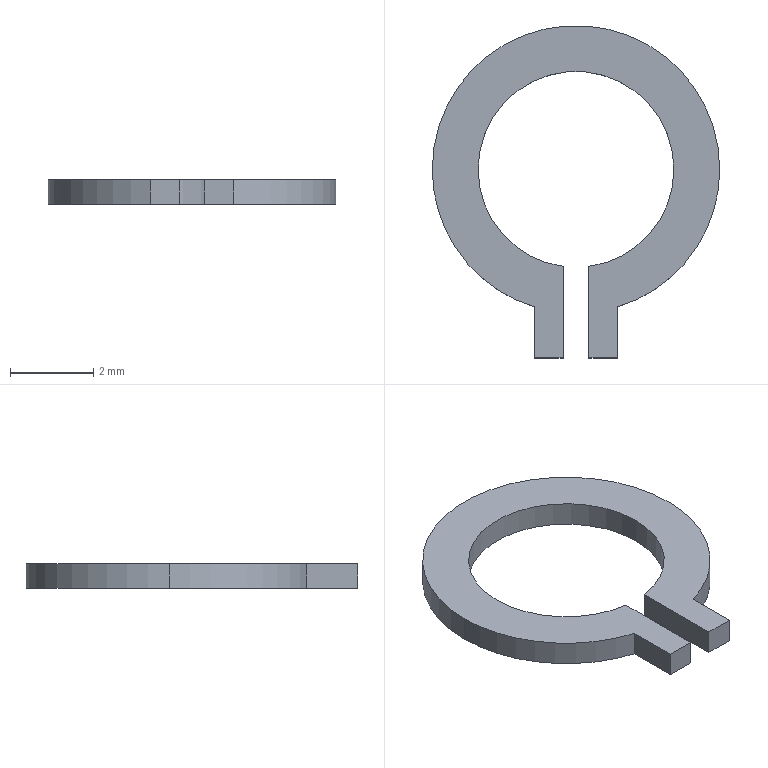Part | NX | 1 solid | 14 faces | box 6.9 x 7.977 x 0.6 mm | volume 12.565 mm3 | plane 8 | cylinder 6 | commonest cylinder face diameters 4.7 x3 6.9 x3
STEP:
#1=CARTESIAN_POINT('',(-1.,-4.527,0.));
#2=VERTEX_POINT('',#1);
#3=CARTESIAN_POINT('',(-1.,-3.302,0.));
#4=VERTEX_POINT('',#3);
#5=CARTESIAN_POINT('',(-1.,-4.527,0.));
#6=DIRECTION('',(0.,1.,0.));
#7=VECTOR('',#6,1000.);
#8=LINE('',#5,#7);
#9=EDGE_CURVE('',#2,#4,#8,.T.);
#10=ORIENTED_EDGE('',*,*,#9,.T.);
#11=CARTESIAN_POINT('',(-3.45,0.,0.));
#12=VERTEX_POINT('',#11);
#13=CARTESIAN_POINT('',(0.,0.,0.));
#14=DIRECTION('',(0.,0.,1.));
#15=DIRECTION('',(-1.,0.,0.));
#16=AXIS2_PLACEMENT_3D('',#13,#14,#15);
#17=CIRCLE('',#16,3.45);
#18=EDGE_CURVE('',#12,#4,#17,.T.);
#19=ORIENTED_EDGE('',*,*,#18,.F.);
#20=CARTESIAN_POINT('',(3.45,0.,0.));
#21=VERTEX_POINT('',#20);
#22=CARTESIAN_POINT('',(0.,0.,0.));
#23=DIRECTION('',(0.,0.,1.));
#24=DIRECTION('',(-1.,0.,0.));
#25=AXIS2_PLACEMENT_3D('',#22,#23,#24);
#26=CIRCLE('',#25,3.45);
#27=EDGE_CURVE('',#21,#12,#26,.T.);
#28=ORIENTED_EDGE('',*,*,#27,.F.);
#29=CARTESIAN_POINT('',(1.,-3.302,0.));
#30=VERTEX_POINT('',#29);
#31=CARTESIAN_POINT('',(0.,0.,0.));
#32=DIRECTION('',(0.,0.,1.));
#33=DIRECTION('',(-1.,0.,0.));
#34=AXIS2_PLACEMENT_3D('',#31,#32,#33);
#35=CIRCLE('',#34,3.45);
#36=EDGE_CURVE('',#30,#21,#35,.T.);
#37=ORIENTED_EDGE('',*,*,#36,.F.);
#38=CARTESIAN_POINT('',(1.,-4.527,0.));
#39=VERTEX_POINT('',#38);
#40=CARTESIAN_POINT('',(1.,-3.302,0.));
#41=DIRECTION('',(0.,-1.,0.));
#42=VECTOR('',#41,1000.);
#43=LINE('',#40,#42);
#44=EDGE_CURVE('',#30,#39,#43,.T.);
#45=ORIENTED_EDGE('',*,*,#44,.T.);
#46=CARTESIAN_POINT('',(0.31,-4.527,0.));
#47=VERTEX_POINT('',#46);
#48=CARTESIAN_POINT('',(1.,-4.527,0.));
#49=DIRECTION('',(-1.,0.,0.));
#50=VECTOR('',#49,1000.);
#51=LINE('',#48,#50);
#52=EDGE_CURVE('',#39,#47,#51,.T.);
#53=ORIENTED_EDGE('',*,*,#52,.T.);
#54=CARTESIAN_POINT('',(0.31,-2.329,0.));
#55=VERTEX_POINT('',#54);
#56=CARTESIAN_POINT('',(0.31,-4.527,0.));
#57=DIRECTION('',(0.,1.,0.));
#58=VECTOR('',#57,1000.);
#59=LINE('',#56,#58);
#60=EDGE_CURVE('',#47,#55,#59,.T.);
#61=ORIENTED_EDGE('',*,*,#60,.T.);
#62=CARTESIAN_POINT('',(2.35,0.,0.));
#63=VERTEX_POINT('',#62);
#64=CARTESIAN_POINT('',(0.,0.,0.));
#65=DIRECTION('',(0.,0.,-1.));
#66=DIRECTION('',(1.,0.,0.));
#67=AXIS2_PLACEMENT_3D('',#64,#65,#66);
#68=CIRCLE('',#67,2.35);
#69=EDGE_CURVE('',#63,#55,#68,.T.);
#70=ORIENTED_EDGE('',*,*,#69,.F.);
#71=CARTESIAN_POINT('',(-2.35,0.,0.));
#72=VERTEX_POINT('',#71);
#73=CARTESIAN_POINT('',(0.,0.,0.));
#74=DIRECTION('',(0.,0.,-1.));
#75=DIRECTION('',(1.,0.,0.));
#76=AXIS2_PLACEMENT_3D('',#73,#74,#75);
#77=CIRCLE('',#76,2.35);
#78=EDGE_CURVE('',#72,#63,#77,.T.);
#79=ORIENTED_EDGE('',*,*,#78,.F.);
#80=CARTESIAN_POINT('',(-0.31,-2.329,0.));
#81=VERTEX_POINT('',#80);
#82=CARTESIAN_POINT('',(0.,0.,0.));
#83=DIRECTION('',(0.,0.,-1.));
#84=DIRECTION('',(1.,0.,0.));
#85=AXIS2_PLACEMENT_3D('',#82,#83,#84);
#86=CIRCLE('',#85,2.35);
#87=EDGE_CURVE('',#81,#72,#86,.T.);
#88=ORIENTED_EDGE('',*,*,#87,.F.);
#89=CARTESIAN_POINT('',(-0.31,-4.527,0.));
#90=VERTEX_POINT('',#89);
#91=CARTESIAN_POINT('',(-0.31,-2.329,0.));
#92=DIRECTION('',(0.,-1.,0.));
#93=VECTOR('',#92,1000.);
#94=LINE('',#91,#93);
#95=EDGE_CURVE('',#81,#90,#94,.T.);
#96=ORIENTED_EDGE('',*,*,#95,.T.);
#97=CARTESIAN_POINT('',(-0.31,-4.527,0.));
#98=DIRECTION('',(-1.,0.,0.));
#99=VECTOR('',#98,1000.);
#100=LINE('',#97,#99);
#101=EDGE_CURVE('',#90,#2,#100,.T.);
#102=ORIENTED_EDGE('',*,*,#101,.T.);
#103=EDGE_LOOP('',(#10,#19,#28,#37,#45,#53,#61,#70,#79,#88,#96,#102));
#104=FACE_BOUND('',#103,.T.);
#105=CARTESIAN_POINT('',(0.,0.,0.));
#106=DIRECTION('',(0.,0.,1.));
#107=DIRECTION('',(1.,0.,0.));
#108=AXIS2_PLACEMENT_3D('',#105,#106,#107);
#109=PLANE('',#108);
#110=ADVANCED_FACE('',(#104),#109,.F.);
#111=ORIENTED_EDGE('',*,*,#9,.F.);
#112=CARTESIAN_POINT('',(-1.,-4.527,0.6));
#113=VERTEX_POINT('',#112);
#114=CARTESIAN_POINT('',(-1.,-4.527,0.6));
#115=DIRECTION('',(0.,0.,-1.));
#116=VECTOR('',#115,1000.);
#117=LINE('',#114,#116);
#118=EDGE_CURVE('',#113,#2,#117,.T.);
#119=ORIENTED_EDGE('',*,*,#118,.F.);
#120=CARTESIAN_POINT('',(-1.,-3.302,0.6));
#121=VERTEX_POINT('',#120);
#122=CARTESIAN_POINT('',(-1.,-4.527,0.6));
#123=DIRECTION('',(0.,1.,0.));
#124=VECTOR('',#123,1000.);
#125=LINE('',#122,#124);
#126=EDGE_CURVE('',#113,#121,#125,.T.);
#127=ORIENTED_EDGE('',*,*,#126,.T.);
#128=CARTESIAN_POINT('',(-1.,-3.302,0.6));
#129=DIRECTION('',(0.,0.,-1.));
#130=VECTOR('',#129,1000.);
#131=LINE('',#128,#130);
#132=EDGE_CURVE('',#121,#4,#131,.T.);
#133=ORIENTED_EDGE('',*,*,#132,.T.);
#134=EDGE_LOOP('',(#111,#119,#127,#133));
#135=FACE_BOUND('',#134,.T.);
#136=CARTESIAN_POINT('',(-1.,-3.302,0.));
#137=DIRECTION('',(-1.,0.,0.));
#138=DIRECTION('',(0.,0.,1.));
#139=AXIS2_PLACEMENT_3D('',#136,#137,#138);
#140=PLANE('',#139);
#141=ADVANCED_FACE('',(#135),#140,.T.);
#142=CARTESIAN_POINT('',(-3.45,0.,0.6));
#143=VERTEX_POINT('',#142);
#144=CARTESIAN_POINT('',(-3.45,0.,0.));
#145=DIRECTION('',(0.,0.,1.));
#146=VECTOR('',#145,1000.);
#147=LINE('',#144,#146);
#148=EDGE_CURVE('',#12,#143,#147,.T.);
#149=ORIENTED_EDGE('',*,*,#148,.F.);
#150=ORIENTED_EDGE('',*,*,#18,.T.);
#151=ORIENTED_EDGE('',*,*,#132,.F.);
#152=CARTESIAN_POINT('',(0.,0.,0.6));
#153=DIRECTION('',(0.,0.,-1.));
#154=DIRECTION('',(-0.2899,-0.9571,0.));
#155=AXIS2_PLACEMENT_3D('',#152,#153,#154);
#156=CIRCLE('',#155,3.45);
#157=EDGE_CURVE('',#121,#143,#156,.T.);
#158=ORIENTED_EDGE('',*,*,#157,.T.);
#159=EDGE_LOOP('',(#149,#150,#151,#158));
#160=FACE_BOUND('',#159,.T.);
#161=CARTESIAN_POINT('',(0.,0.,0.));
#162=DIRECTION('',(0.,0.,1.));
#163=DIRECTION('',(1.,0.,0.));
#164=AXIS2_PLACEMENT_3D('',#161,#162,#163);
#165=CYLINDRICAL_SURFACE('',#164,3.45);
#166=ADVANCED_FACE('',(#160),#165,.T.);
#167=ORIENTED_EDGE('',*,*,#44,.F.);
#168=CARTESIAN_POINT('',(1.,-3.302,0.6));
#169=VERTEX_POINT('',#168);
#170=CARTESIAN_POINT('',(1.,-3.302,0.));
#171=DIRECTION('',(0.,0.,1.));
#172=VECTOR('',#171,1000.);
#173=LINE('',#170,#172);
#174=EDGE_CURVE('',#30,#169,#173,.T.);
#175=ORIENTED_EDGE('',*,*,#174,.T.);
#176=CARTESIAN_POINT('',(1.,-4.527,0.6));
#177=VERTEX_POINT('',#176);
#178=CARTESIAN_POINT('',(1.,-3.302,0.6));
#179=DIRECTION('',(0.,-1.,0.));
#180=VECTOR('',#179,1000.);
#181=LINE('',#178,#180);
#182=EDGE_CURVE('',#169,#177,#181,.T.);
#183=ORIENTED_EDGE('',*,*,#182,.T.);
#184=CARTESIAN_POINT('',(1.,-4.527,0.6));
#185=DIRECTION('',(0.,0.,-1.));
#186=VECTOR('',#185,1000.);
#187=LINE('',#184,#186);
#188=EDGE_CURVE('',#177,#39,#187,.T.);
#189=ORIENTED_EDGE('',*,*,#188,.T.);
#190=EDGE_LOOP('',(#167,#175,#183,#189));
#191=FACE_BOUND('',#190,.T.);
#192=CARTESIAN_POINT('',(1.,-4.527,0.));
#193=DIRECTION('',(1.,0.,0.));
#194=DIRECTION('',(0.,1.,0.));
#195=AXIS2_PLACEMENT_3D('',#192,#193,#194);
#196=PLANE('',#195);
#197=ADVANCED_FACE('',(#191),#196,.T.);
#198=ORIENTED_EDGE('',*,*,#52,.F.);
#199=ORIENTED_EDGE('',*,*,#188,.F.);
#200=CARTESIAN_POINT('',(0.31,-4.527,0.6));
#201=VERTEX_POINT('',#200);
#202=CARTESIAN_POINT('',(1.,-4.527,0.6));
#203=DIRECTION('',(-1.,0.,0.));
#204=VECTOR('',#203,1000.);
#205=LINE('',#202,#204);
#206=EDGE_CURVE('',#177,#201,#205,.T.);
#207=ORIENTED_EDGE('',*,*,#206,.T.);
#208=CARTESIAN_POINT('',(0.31,-4.527,0.6));
#209=DIRECTION('',(0.,0.,-1.));
#210=VECTOR('',#209,1000.);
#211=LINE('',#208,#210);
#212=EDGE_CURVE('',#201,#47,#211,.T.);
#213=ORIENTED_EDGE('',*,*,#212,.T.);
#214=EDGE_LOOP('',(#198,#199,#207,#213));
#215=FACE_BOUND('',#214,.T.);
#216=CARTESIAN_POINT('',(0.31,-4.527,0.));
#217=DIRECTION('',(0.,-1.,0.));
#218=DIRECTION('',(0.,0.,-1.));
#219=AXIS2_PLACEMENT_3D('',#216,#217,#218);
#220=PLANE('',#219);
#221=ADVANCED_FACE('',(#215),#220,.T.);
#222=ORIENTED_EDGE('',*,*,#60,.F.);
#223=ORIENTED_EDGE('',*,*,#212,.F.);
#224=CARTESIAN_POINT('',(0.31,-2.329,0.6));
#225=VERTEX_POINT('',#224);
#226=CARTESIAN_POINT('',(0.31,-4.527,0.6));
#227=DIRECTION('',(0.,1.,0.));
#228=VECTOR('',#227,1000.);
#229=LINE('',#226,#228);
#230=EDGE_CURVE('',#201,#225,#229,.T.);
#231=ORIENTED_EDGE('',*,*,#230,.T.);
#232=CARTESIAN_POINT('',(0.31,-2.329,0.6));
#233=DIRECTION('',(0.,0.,-1.));
#234=VECTOR('',#233,1000.);
#235=LINE('',#232,#234);
#236=EDGE_CURVE('',#225,#55,#235,.T.);
#237=ORIENTED_EDGE('',*,*,#236,.T.);
#238=EDGE_LOOP('',(#222,#223,#231,#237));
#239=FACE_BOUND('',#238,.T.);
#240=CARTESIAN_POINT('',(0.31,-2.329,0.));
#241=DIRECTION('',(-1.,0.,0.));
#242=DIRECTION('',(0.,0.,1.));
#243=AXIS2_PLACEMENT_3D('',#240,#241,#242);
#244=PLANE('',#243);
#245=ADVANCED_FACE('',(#239),#244,.T.);
#246=CARTESIAN_POINT('',(2.35,0.,0.6));
#247=VERTEX_POINT('',#246);
#248=CARTESIAN_POINT('',(2.35,0.,0.));
#249=DIRECTION('',(0.,0.,1.));
#250=VECTOR('',#249,1000.);
#251=LINE('',#248,#250);
#252=EDGE_CURVE('',#63,#247,#251,.T.);
#253=ORIENTED_EDGE('',*,*,#252,.F.);
#254=ORIENTED_EDGE('',*,*,#69,.T.);
#255=ORIENTED_EDGE('',*,*,#236,.F.);
#256=CARTESIAN_POINT('',(0.,0.,0.6));
#257=DIRECTION('',(0.,0.,1.));
#258=DIRECTION('',(0.1319,-0.9913,0.));
#259=AXIS2_PLACEMENT_3D('',#256,#257,#258);
#260=CIRCLE('',#259,2.35);
#261=EDGE_CURVE('',#225,#247,#260,.T.);
#262=ORIENTED_EDGE('',*,*,#261,.T.);
#263=EDGE_LOOP('',(#253,#254,#255,#262));
#264=FACE_BOUND('',#263,.T.);
#265=CARTESIAN_POINT('',(0.,0.,0.));
#266=DIRECTION('',(0.,0.,1.));
#267=DIRECTION('',(1.,0.,0.));
#268=AXIS2_PLACEMENT_3D('',#265,#266,#267);
#269=CYLINDRICAL_SURFACE('',#268,2.35);
#270=ADVANCED_FACE('',(#264),#269,.F.);
#271=ORIENTED_EDGE('',*,*,#95,.F.);
#272=CARTESIAN_POINT('',(-0.31,-2.329,0.6));
#273=VERTEX_POINT('',#272);
#274=CARTESIAN_POINT('',(-0.31,-2.329,0.));
#275=DIRECTION('',(0.,0.,1.));
#276=VECTOR('',#275,1000.);
#277=LINE('',#274,#276);
#278=EDGE_CURVE('',#81,#273,#277,.T.);
#279=ORIENTED_EDGE('',*,*,#278,.T.);
#280=CARTESIAN_POINT('',(-0.31,-4.527,0.6));
#281=VERTEX_POINT('',#280);
#282=CARTESIAN_POINT('',(-0.31,-2.329,0.6));
#283=DIRECTION('',(0.,-1.,0.));
#284=VECTOR('',#283,1000.);
#285=LINE('',#282,#284);
#286=EDGE_CURVE('',#273,#281,#285,.T.);
#287=ORIENTED_EDGE('',*,*,#286,.T.);
#288=CARTESIAN_POINT('',(-0.31,-4.527,0.6));
#289=DIRECTION('',(0.,0.,-1.));
#290=VECTOR('',#289,1000.);
#291=LINE('',#288,#290);
#292=EDGE_CURVE('',#281,#90,#291,.T.);
#293=ORIENTED_EDGE('',*,*,#292,.T.);
#294=EDGE_LOOP('',(#271,#279,#287,#293));
#295=FACE_BOUND('',#294,.T.);
#296=CARTESIAN_POINT('',(-0.31,-4.527,0.));
#297=DIRECTION('',(1.,0.,0.));
#298=DIRECTION('',(0.,1.,0.));
#299=AXIS2_PLACEMENT_3D('',#296,#297,#298);
#300=PLANE('',#299);
#301=ADVANCED_FACE('',(#295),#300,.T.);
#302=ORIENTED_EDGE('',*,*,#101,.F.);
#303=ORIENTED_EDGE('',*,*,#292,.F.);
#304=CARTESIAN_POINT('',(-0.31,-4.527,0.6));
#305=DIRECTION('',(-1.,0.,0.));
#306=VECTOR('',#305,1000.);
#307=LINE('',#304,#306);
#308=EDGE_CURVE('',#281,#113,#307,.T.);
#309=ORIENTED_EDGE('',*,*,#308,.T.);
#310=ORIENTED_EDGE('',*,*,#118,.T.);
#311=EDGE_LOOP('',(#302,#303,#309,#310));
#312=FACE_BOUND('',#311,.T.);
#313=CARTESIAN_POINT('',(-1.,-4.527,0.));
#314=DIRECTION('',(0.,-1.,0.));
#315=DIRECTION('',(0.,0.,-1.));
#316=AXIS2_PLACEMENT_3D('',#313,#314,#315);
#317=PLANE('',#316);
#318=ADVANCED_FACE('',(#312),#317,.T.);
#319=ORIENTED_EDGE('',*,*,#126,.F.);
#320=ORIENTED_EDGE('',*,*,#308,.F.);
#321=ORIENTED_EDGE('',*,*,#286,.F.);
#322=CARTESIAN_POINT('',(-2.35,0.,0.6));
#323=VERTEX_POINT('',#322);
#324=CARTESIAN_POINT('',(0.,0.,0.6));
#325=DIRECTION('',(0.,0.,1.));
#326=DIRECTION('',(0.1319,-0.9913,0.));
#327=AXIS2_PLACEMENT_3D('',#324,#325,#326);
#328=CIRCLE('',#327,2.35);
#329=EDGE_CURVE('',#323,#273,#328,.T.);
#330=ORIENTED_EDGE('',*,*,#329,.F.);
#331=CARTESIAN_POINT('',(0.,0.,0.6));
#332=DIRECTION('',(0.,0.,1.));
#333=DIRECTION('',(0.1319,-0.9913,0.));
#334=AXIS2_PLACEMENT_3D('',#331,#332,#333);
#335=CIRCLE('',#334,2.35);
#336=EDGE_CURVE('',#247,#323,#335,.T.);
#337=ORIENTED_EDGE('',*,*,#336,.F.);
#338=ORIENTED_EDGE('',*,*,#261,.F.);
#339=ORIENTED_EDGE('',*,*,#230,.F.);
#340=ORIENTED_EDGE('',*,*,#206,.F.);
#341=ORIENTED_EDGE('',*,*,#182,.F.);
#342=CARTESIAN_POINT('',(3.45,0.,0.6));
#343=VERTEX_POINT('',#342);
#344=CARTESIAN_POINT('',(0.,0.,0.6));
#345=DIRECTION('',(0.,0.,-1.));
#346=DIRECTION('',(-0.2899,-0.9571,0.));
#347=AXIS2_PLACEMENT_3D('',#344,#345,#346);
#348=CIRCLE('',#347,3.45);
#349=EDGE_CURVE('',#343,#169,#348,.T.);
#350=ORIENTED_EDGE('',*,*,#349,.F.);
#351=CARTESIAN_POINT('',(0.,0.,0.6));
#352=DIRECTION('',(0.,0.,-1.));
#353=DIRECTION('',(-0.2899,-0.9571,0.));
#354=AXIS2_PLACEMENT_3D('',#351,#352,#353);
#355=CIRCLE('',#354,3.45);
#356=EDGE_CURVE('',#143,#343,#355,.T.);
#357=ORIENTED_EDGE('',*,*,#356,.F.);
#358=ORIENTED_EDGE('',*,*,#157,.F.);
#359=EDGE_LOOP('',(#319,#320,#321,#330,#337,#338,#339,#340,#341,#350,#357,#358));
#360=FACE_BOUND('',#359,.T.);
#361=CARTESIAN_POINT('',(0.,0.,0.6));
#362=DIRECTION('',(0.,0.,1.));
#363=DIRECTION('',(1.,0.,0.));
#364=AXIS2_PLACEMENT_3D('',#361,#362,#363);
#365=PLANE('',#364);
#366=ADVANCED_FACE('',(#360),#365,.T.);
#367=CARTESIAN_POINT('',(-2.35,0.,0.));
#368=DIRECTION('',(0.,0.,1.));
#369=VECTOR('',#368,1000.);
#370=LINE('',#367,#369);
#371=EDGE_CURVE('',#72,#323,#370,.T.);
#372=ORIENTED_EDGE('',*,*,#371,.F.);
#373=ORIENTED_EDGE('',*,*,#78,.T.);
#374=ORIENTED_EDGE('',*,*,#252,.T.);
#375=ORIENTED_EDGE('',*,*,#336,.T.);
#376=EDGE_LOOP('',(#372,#373,#374,#375));
#377=FACE_BOUND('',#376,.T.);
#378=CARTESIAN_POINT('',(0.,0.,0.));
#379=DIRECTION('',(0.,0.,1.));
#380=DIRECTION('',(1.,0.,0.));
#381=AXIS2_PLACEMENT_3D('',#378,#379,#380);
#382=CYLINDRICAL_SURFACE('',#381,2.35);
#383=ADVANCED_FACE('',(#377),#382,.F.);
#384=ORIENTED_EDGE('',*,*,#87,.T.);
#385=ORIENTED_EDGE('',*,*,#371,.T.);
#386=ORIENTED_EDGE('',*,*,#329,.T.);
#387=ORIENTED_EDGE('',*,*,#278,.F.);
#388=EDGE_LOOP('',(#384,#385,#386,#387));
#389=FACE_BOUND('',#388,.T.);
#390=CARTESIAN_POINT('',(0.,0.,0.));
#391=DIRECTION('',(0.,0.,1.));
#392=DIRECTION('',(1.,0.,0.));
#393=AXIS2_PLACEMENT_3D('',#390,#391,#392);
#394=CYLINDRICAL_SURFACE('',#393,2.35);
#395=ADVANCED_FACE('',(#389),#394,.F.);
#396=ORIENTED_EDGE('',*,*,#36,.T.);
#397=CARTESIAN_POINT('',(3.45,0.,0.));
#398=DIRECTION('',(0.,0.,1.));
#399=VECTOR('',#398,1000.);
#400=LINE('',#397,#399);
#401=EDGE_CURVE('',#21,#343,#400,.T.);
#402=ORIENTED_EDGE('',*,*,#401,.T.);
#403=ORIENTED_EDGE('',*,*,#349,.T.);
#404=ORIENTED_EDGE('',*,*,#174,.F.);
#405=EDGE_LOOP('',(#396,#402,#403,#404));
#406=FACE_BOUND('',#405,.T.);
#407=CARTESIAN_POINT('',(0.,0.,0.));
#408=DIRECTION('',(0.,0.,1.));
#409=DIRECTION('',(1.,0.,0.));
#410=AXIS2_PLACEMENT_3D('',#407,#408,#409);
#411=CYLINDRICAL_SURFACE('',#410,3.45);
#412=ADVANCED_FACE('',(#406),#411,.T.);
#413=ORIENTED_EDGE('',*,*,#27,.T.);
#414=ORIENTED_EDGE('',*,*,#148,.T.);
#415=ORIENTED_EDGE('',*,*,#356,.T.);
#416=ORIENTED_EDGE('',*,*,#401,.F.);
#417=EDGE_LOOP('',(#413,#414,#415,#416));
#418=FACE_BOUND('',#417,.T.);
#419=CARTESIAN_POINT('',(0.,0.,0.));
#420=DIRECTION('',(0.,0.,1.));
#421=DIRECTION('',(1.,0.,0.));
#422=AXIS2_PLACEMENT_3D('',#419,#420,#421);
#423=CYLINDRICAL_SURFACE('',#422,3.45);
#424=ADVANCED_FACE('',(#418),#423,.T.);
#425=CLOSED_SHELL('',(#110,#141,#166,#197,#221,#245,#270,#301,#318,#366,#383,#395,#412,#424));
#426=MANIFOLD_SOLID_BREP('',#425);
#427=(LENGTH_UNIT()NAMED_UNIT(*)SI_UNIT(.MILLI.,.METRE.));
#428=UNCERTAINTY_MEASURE_WITH_UNIT(LENGTH_MEASURE(0.00001),#427,'','');
#429=(NAMED_UNIT(*)PLANE_ANGLE_UNIT()SI_UNIT($,.RADIAN.));
#430=(NAMED_UNIT(*)SI_UNIT($,.STERADIAN.)SOLID_ANGLE_UNIT());
#431=(GEOMETRIC_REPRESENTATION_CONTEXT(3)GLOBAL_UNCERTAINTY_ASSIGNED_CONTEXT((#428))GLOBAL_UNIT_ASSIGNED_CONTEXT((#427,#429,#430))REPRESENTATION_CONTEXT('',''));
#432=ADVANCED_BREP_SHAPE_REPRESENTATION('',(#426),#431);